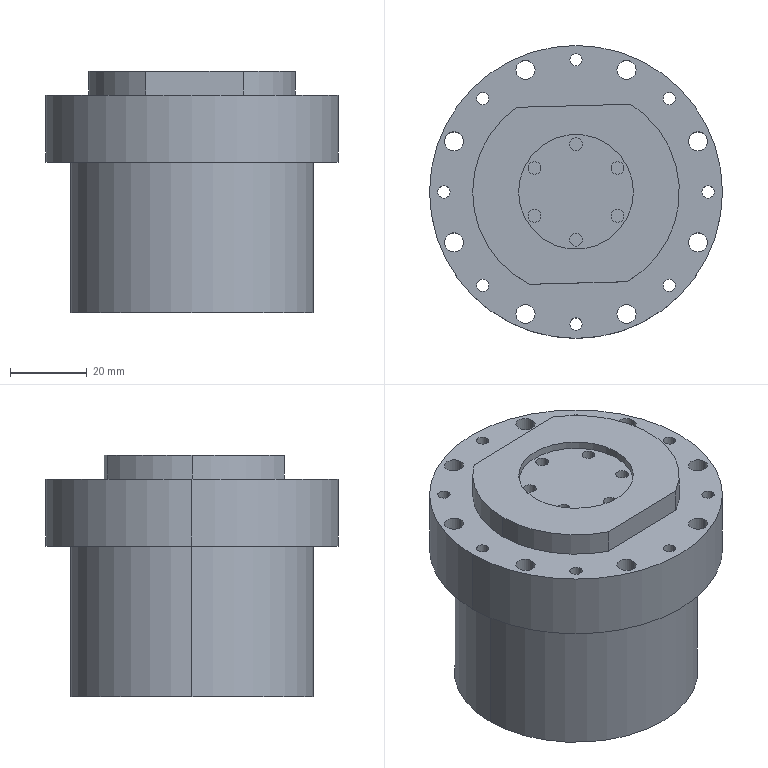Part | SolidWorks | features ICE 3, Extrusion 1 | 1 solid | 66 faces | box 76.5 x 76.5 x 63 mm | volume 212682 mm3 | cylinder 53 | plane 13 | commonest cylinder face diameters 3.2 x16 5 x16 3.32 x12 54 x3 30 x2 63.5 x2